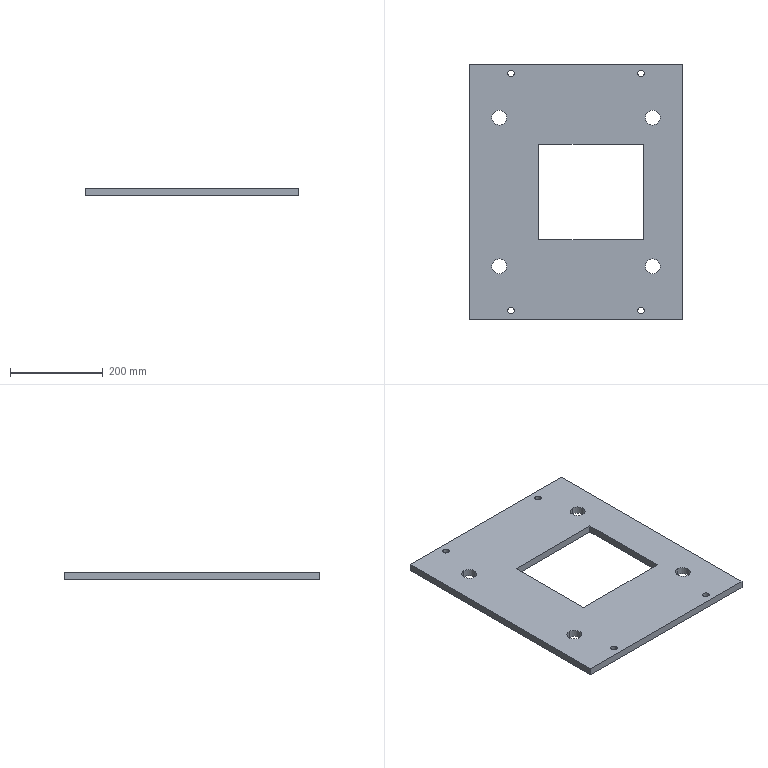Part | STEP file | 02-Top plate | 1 solid | 26 faces | box 460 x 550 x 16 mm | volume 3248676 mm3 | cylinder 16 | plane 10 | commonest cylinder face diameters 14 x8 32 x8